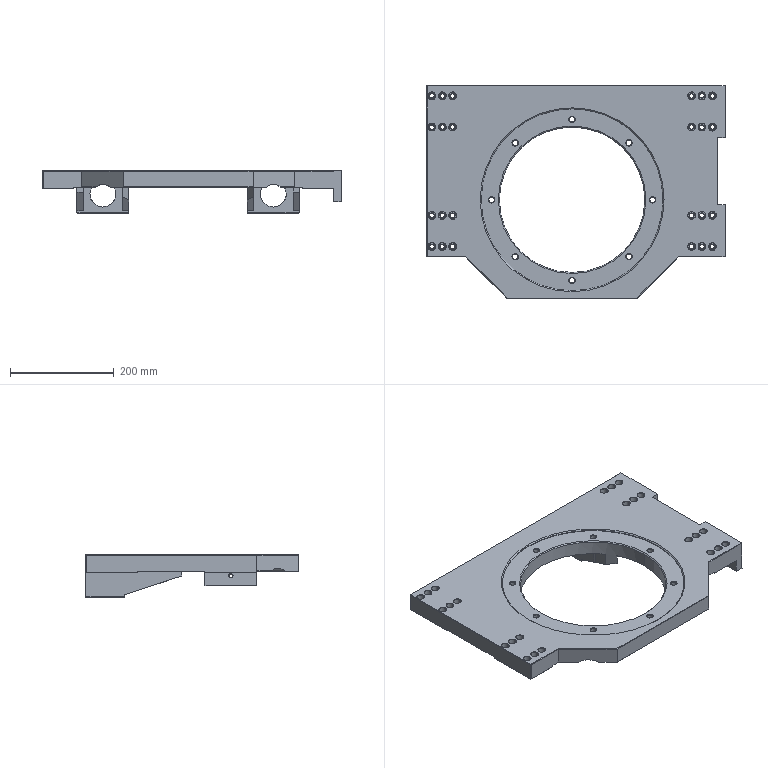Part | SolidWorks | features BaseBody 1 | 1 solid | 501 faces | box 575 x 410 x 82 mm | volume 5326767 mm3 | cone 211 | cylinder 156 | plane 132 | spline 2 | commonest cylinder face diameters 8.5 x48 14 x48 6.5 x28 10.5 x16 1.8 x4 38 x4